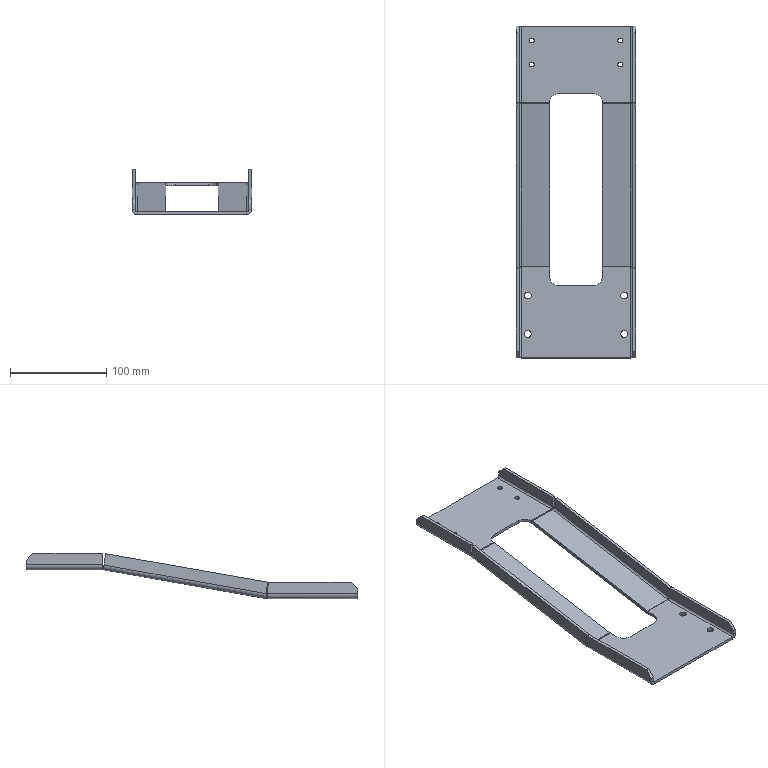Part | SolidWorks | features Chamfer 1, EdgeFlange 1, FlatPattern 1, Jog 1, SMBaseFlange 1, SheetMetal 1 | 1 solid | 112 faces | box 124 x 345 x 47 mm | volume 120902 mm3 | plane 66 | cylinder 40 | spline 6 | commonest cylinder face diameters 5 x8 7 x8 4 x6 10 x6 6 x4 12 x4